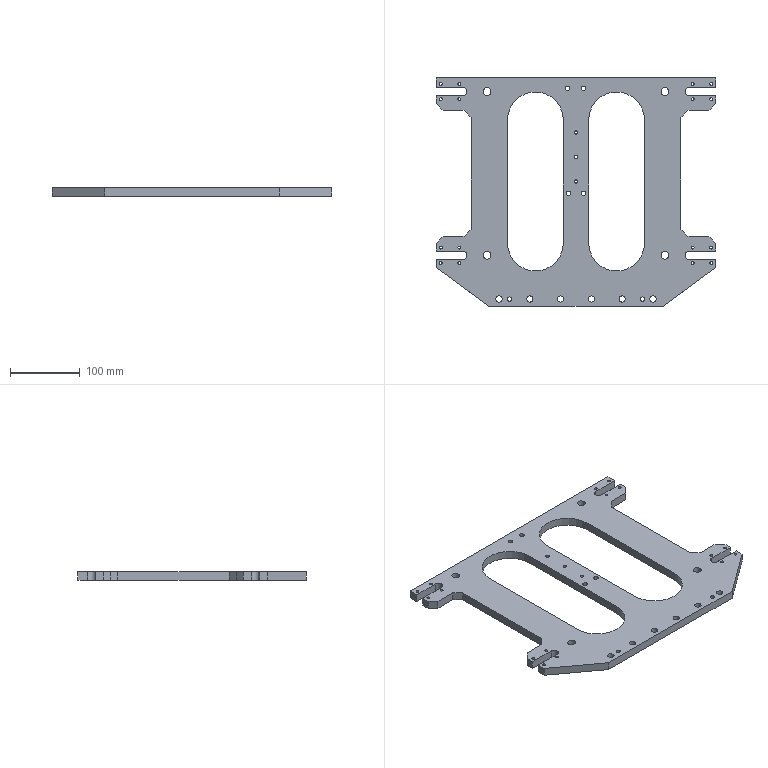CAM job | NX | 3-axis milling, drilling | part box 400 x 326 x 12 mm | stock box 404 x 330 x 12 mm
Tools:
number,name,description,diameter,corner_radius,flute_length,length,flutes
11,ZXZ,Milling Tool-5 Parameters,6.0,0.0,50.0,75.0,2
16,6.0ZT,Drilling Tool,6.0,0.0,35.0,50.0,2
15,5.0ZT,Drilling Tool,5.0,0.0,35.0,50.0,2
17,6.6ZT,Drilling Tool,6.6,0.0,35.0,50.0,2
14,4.2ZT,Drilling Tool,4.2,0.0,35.0,50.0,2
19,9.0ZT,Drilling Tool,9.0,0.0,35.0,50.0,2
12,11.0ZT,Drilling Tool,11.0,0.0,35.0,50.0,2
10,D10,Milling Tool-5 Parameters,10.0,0.0,50.0,75.0,2
9,D10JING,Milling Tool-5 Parameters,10.0,0.0,50.0,75.0,2
6,D6,Milling Tool-5 Parameters,6.0,0.0,50.0,75.0,2
7,D6A45,Milling Tool-5 Parameters,6.0,0.0,3.0,3.0,2
Operations:
program,operation,operation_type,tool,method,geometry_group,spindle_rpm,surface_speed,feed_per_tooth,feed_cut,feed_plunge,cut_length_mm,path_length_mm,cut_time_min,machine_time_min
1压左右,DRILLING,Operation,ZXZ,METHOD,A,3000.0,56.0,0.0417,250.0,0.0,140.0,2032.138,0.56,0.7492
1压左右,DRILLING_COPY,Operation,6.0ZT,METHOD,A,2000.0,37.0,0.045,180.0,0.0,36.605,426.234,0.2034,0.2423
1压左右,DRILLING_COPY_COPY_3,Operation,5.0ZT,METHOD,A,2000.0,37.0,0.045,180.0,0.0,54.007,344.27,0.3,0.3291
1压左右,DRILLING_COPY_COPY_2,Operation,6.6ZT,METHOD,A,2000.0,37.0,0.045,180.0,0.0,73.931,511.994,0.4107,0.4545
1压左右,DRILLING_COPY_COPY_1,Operation,4.2ZT,METHOD,A,2000.0,37.0,0.045,180.0,0.0,284.189,1815.537,1.579,1.732
1压左右,DRILLING_COPY_COPY,Operation,9.0ZT,METHOD,A,1000.0,28.0,0.09,180.0,0.0,115.223,625.957,0.6401,0.6912
1压左右,DRILLING_COPY_COPY_COPY,Operation,11.0ZT,METHOD,A,1000.0,28.0,0.09,180.0,0.0,79.219,1140.847,0.4401,0.5463
1压左右,ZLEVEL_PROFILE,ZLevelMilling,D10,METHOD,A,2200.0,69.0,0.5,2200.0,100.0,49396.3,50035.926,22.453,22.517
1压左右,ZLEVEL_PROFILE_COPY_1,ZLevelMilling,D10,METHOD,A,2200.0,69.0,0.5,2200.0,100.0,61758.708,62283.207,28.072,28.125
1压左右,ZLEVEL_PROFILE_COPY,ZLevelMilling,D10JING,METHOD,A,5000.0,157.0,0.12,1200.0,100.0,876.934,1519.239,0.7308,0.795
1压左右,ZLEVEL_PROFILE_COPY_COPY_1,ZLevelMilling,D6,METHOD,A,5000.0,157.0,0.12,1200.0,100.0,1182.043,1796.545,0.985,1.046
1压左右,ZLEVEL_PROFILE_COPY_COPY,ZLevelMilling,D6A45,METHOD,A,7500.0,141.0,0.08,1200.0,100.0,2857.248,16160.735,2.381,3.711
2压前后,ZLEVEL_PROFILE_COPY_1_1,ZLevelMilling,D10,METHOD,A,2200.0,69.0,0.5,2200.0,100.0,59402.702,60178.261,27.001,27.079
2压前后,ZLEVEL_PROFILE_COPY_COPY_1_1,ZLevelMilling,D10JING,METHOD,A,5000.0,157.0,0.12,1200.0,100.0,1059.41,1834.38,0.8828,0.9603
2压前后,ZLEVEL_PROFILE_COPY_COPY_COPY,ZLevelMilling,D6A45,METHOD,A,7500.0,141.0,0.08,1200.0,100.0,1050.601,1766.428,0.8755,0.9471